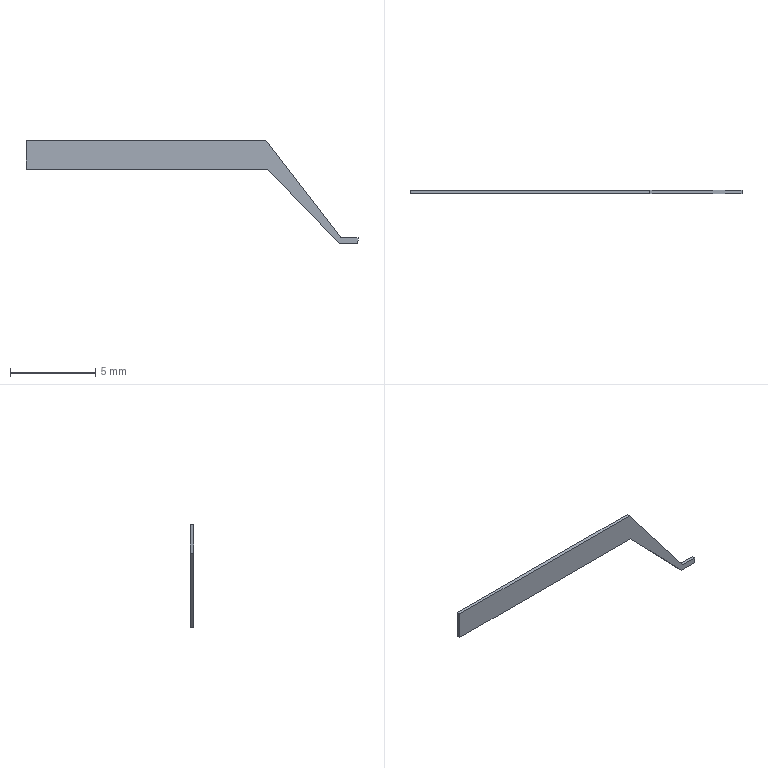Part | SolidWorks | features Extrusion 1 | 1 solid | 10 faces | box 19.5 x 0.2 x 6.07 mm | volume 5.761 mm3 | plane 10
STEP:
#1=CARTESIAN_POINT('',(0.,0.,-1.7));
#2=VERTEX_POINT('',#1);
#3=CARTESIAN_POINT('',(0.,0.,0.));
#4=VERTEX_POINT('',#3);
#5=CARTESIAN_POINT('',(0.,0.,0.));
#6=DIRECTION('',(0.,0.,1.));
#7=VECTOR('',#6,1000.);
#8=LINE('',#5,#7);
#9=EDGE_CURVE('',#2,#4,#8,.T.);
#10=ORIENTED_EDGE('',*,*,#9,.T.);
#11=CARTESIAN_POINT('',(0.,0.2,0.));
#12=VERTEX_POINT('',#11);
#13=CARTESIAN_POINT('',(0.,0.2,0.));
#14=DIRECTION('',(0.,-1.,0.));
#15=VECTOR('',#14,1000.);
#16=LINE('',#13,#15);
#17=EDGE_CURVE('',#12,#4,#16,.T.);
#18=ORIENTED_EDGE('',*,*,#17,.F.);
#19=CARTESIAN_POINT('',(0.,0.2,-1.7));
#20=VERTEX_POINT('',#19);
#21=CARTESIAN_POINT('',(0.,0.2,0.));
#22=DIRECTION('',(0.,0.,1.));
#23=VECTOR('',#22,1000.);
#24=LINE('',#21,#23);
#25=EDGE_CURVE('',#20,#12,#24,.T.);
#26=ORIENTED_EDGE('',*,*,#25,.F.);
#27=CARTESIAN_POINT('',(0.,0.2,-1.7));
#28=DIRECTION('',(0.,-1.,0.));
#29=VECTOR('',#28,1000.);
#30=LINE('',#27,#29);
#31=EDGE_CURVE('',#20,#2,#30,.T.);
#32=ORIENTED_EDGE('',*,*,#31,.T.);
#33=EDGE_LOOP('',(#10,#18,#26,#32));
#34=FACE_OUTER_BOUND('',#33,.T.);
#35=CARTESIAN_POINT('',(0.,0.2,0.));
#36=DIRECTION('',(1.,0.,0.));
#37=DIRECTION('',(0.,0.,-1.));
#38=AXIS2_PLACEMENT_3D('',#35,#36,#37);
#39=PLANE('',#38);
#40=ADVANCED_FACE('',(#34),#39,.F.);
#41=CARTESIAN_POINT('',(14.095,0.,0.));
#42=VERTEX_POINT('',#41);
#43=CARTESIAN_POINT('',(0.,0.,0.));
#44=DIRECTION('',(1.,0.,0.));
#45=VECTOR('',#44,1000.);
#46=LINE('',#43,#45);
#47=EDGE_CURVE('',#4,#42,#46,.T.);
#48=ORIENTED_EDGE('',*,*,#47,.T.);
#49=CARTESIAN_POINT('',(14.095,0.2,0.));
#50=VERTEX_POINT('',#49);
#51=CARTESIAN_POINT('',(14.095,0.2,0.));
#52=DIRECTION('',(0.,-1.,0.));
#53=VECTOR('',#52,1000.);
#54=LINE('',#51,#53);
#55=EDGE_CURVE('',#50,#42,#54,.T.);
#56=ORIENTED_EDGE('',*,*,#55,.F.);
#57=CARTESIAN_POINT('',(0.,0.2,0.));
#58=DIRECTION('',(1.,0.,0.));
#59=VECTOR('',#58,1000.);
#60=LINE('',#57,#59);
#61=EDGE_CURVE('',#12,#50,#60,.T.);
#62=ORIENTED_EDGE('',*,*,#61,.F.);
#63=ORIENTED_EDGE('',*,*,#17,.T.);
#64=EDGE_LOOP('',(#48,#56,#62,#63));
#65=FACE_OUTER_BOUND('',#64,.T.);
#66=CARTESIAN_POINT('',(0.,0.2,0.));
#67=DIRECTION('',(0.,0.,-1.));
#68=DIRECTION('',(-1.,0.,0.));
#69=AXIS2_PLACEMENT_3D('',#66,#67,#68);
#70=PLANE('',#69);
#71=ADVANCED_FACE('',(#65),#70,.F.);
#72=CARTESIAN_POINT('',(18.5,0.,-5.72));
#73=VERTEX_POINT('',#72);
#74=CARTESIAN_POINT('',(14.095,0.,0.));
#75=DIRECTION('',(0.6101,0.,-0.7923));
#76=VECTOR('',#75,1000.);
#77=LINE('',#74,#76);
#78=EDGE_CURVE('',#42,#73,#77,.T.);
#79=ORIENTED_EDGE('',*,*,#78,.T.);
#80=CARTESIAN_POINT('',(18.5,0.2,-5.72));
#81=VERTEX_POINT('',#80);
#82=CARTESIAN_POINT('',(18.5,0.2,-5.72));
#83=DIRECTION('',(0.,-1.,0.));
#84=VECTOR('',#83,1000.);
#85=LINE('',#82,#84);
#86=EDGE_CURVE('',#81,#73,#85,.T.);
#87=ORIENTED_EDGE('',*,*,#86,.F.);
#88=CARTESIAN_POINT('',(14.095,0.2,0.));
#89=DIRECTION('',(0.6101,0.,-0.7923));
#90=VECTOR('',#89,1000.);
#91=LINE('',#88,#90);
#92=EDGE_CURVE('',#50,#81,#91,.T.);
#93=ORIENTED_EDGE('',*,*,#92,.F.);
#94=ORIENTED_EDGE('',*,*,#55,.T.);
#95=EDGE_LOOP('',(#79,#87,#93,#94));
#96=FACE_OUTER_BOUND('',#95,.T.);
#97=CARTESIAN_POINT('',(14.095,0.2,0.));
#98=DIRECTION('',(-0.7923,0.,-0.6101));
#99=DIRECTION('',(-0.6101,0.,0.7923));
#100=AXIS2_PLACEMENT_3D('',#97,#98,#99);
#101=PLANE('',#100);
#102=ADVANCED_FACE('',(#96),#101,.F.);
#103=CARTESIAN_POINT('',(19.5,0.,-5.72));
#104=VERTEX_POINT('',#103);
#105=CARTESIAN_POINT('',(18.5,0.,-5.72));
#106=DIRECTION('',(1.,0.,0.));
#107=VECTOR('',#106,1000.);
#108=LINE('',#105,#107);
#109=EDGE_CURVE('',#73,#104,#108,.T.);
#110=ORIENTED_EDGE('',*,*,#109,.T.);
#111=CARTESIAN_POINT('',(19.5,0.2,-5.72));
#112=VERTEX_POINT('',#111);
#113=CARTESIAN_POINT('',(19.5,0.2,-5.72));
#114=DIRECTION('',(0.,-1.,0.));
#115=VECTOR('',#114,1000.);
#116=LINE('',#113,#115);
#117=EDGE_CURVE('',#112,#104,#116,.T.);
#118=ORIENTED_EDGE('',*,*,#117,.F.);
#119=CARTESIAN_POINT('',(18.5,0.2,-5.72));
#120=DIRECTION('',(1.,0.,0.));
#121=VECTOR('',#120,1000.);
#122=LINE('',#119,#121);
#123=EDGE_CURVE('',#81,#112,#122,.T.);
#124=ORIENTED_EDGE('',*,*,#123,.F.);
#125=ORIENTED_EDGE('',*,*,#86,.T.);
#126=EDGE_LOOP('',(#110,#118,#124,#125));
#127=FACE_OUTER_BOUND('',#126,.T.);
#128=CARTESIAN_POINT('',(18.5,0.2,-5.72));
#129=DIRECTION('',(0.,0.,-1.));
#130=DIRECTION('',(-1.,0.,0.));
#131=AXIS2_PLACEMENT_3D('',#128,#129,#130);
#132=PLANE('',#131);
#133=ADVANCED_FACE('',(#127),#132,.F.);
#134=CARTESIAN_POINT('',(19.5,0.,-6.07));
#135=VERTEX_POINT('',#134);
#136=CARTESIAN_POINT('',(19.5,0.,-5.72));
#137=DIRECTION('',(0.,0.,-1.));
#138=VECTOR('',#137,1000.);
#139=LINE('',#136,#138);
#140=EDGE_CURVE('',#104,#135,#139,.T.);
#141=ORIENTED_EDGE('',*,*,#140,.T.);
#142=CARTESIAN_POINT('',(19.5,0.2,-6.07));
#143=VERTEX_POINT('',#142);
#144=CARTESIAN_POINT('',(19.5,0.2,-6.07));
#145=DIRECTION('',(0.,-1.,0.));
#146=VECTOR('',#145,1000.);
#147=LINE('',#144,#146);
#148=EDGE_CURVE('',#143,#135,#147,.T.);
#149=ORIENTED_EDGE('',*,*,#148,.F.);
#150=CARTESIAN_POINT('',(19.5,0.2,-5.72));
#151=DIRECTION('',(0.,0.,-1.));
#152=VECTOR('',#151,1000.);
#153=LINE('',#150,#152);
#154=EDGE_CURVE('',#112,#143,#153,.T.);
#155=ORIENTED_EDGE('',*,*,#154,.F.);
#156=ORIENTED_EDGE('',*,*,#117,.T.);
#157=EDGE_LOOP('',(#141,#149,#155,#156));
#158=FACE_OUTER_BOUND('',#157,.T.);
#159=CARTESIAN_POINT('',(19.5,0.2,-5.72));
#160=DIRECTION('',(-1.,0.,0.));
#161=DIRECTION('',(0.,0.,1.));
#162=AXIS2_PLACEMENT_3D('',#159,#160,#161);
#163=PLANE('',#162);
#164=ADVANCED_FACE('',(#158),#163,.F.);
#165=CARTESIAN_POINT('',(18.405,0.,-6.07));
#166=VERTEX_POINT('',#165);
#167=CARTESIAN_POINT('',(18.405,0.,-6.07));
#168=DIRECTION('',(-1.,0.,0.));
#169=VECTOR('',#168,1000.);
#170=LINE('',#167,#169);
#171=EDGE_CURVE('',#135,#166,#170,.T.);
#172=ORIENTED_EDGE('',*,*,#171,.T.);
#173=CARTESIAN_POINT('',(18.405,0.2,-6.07));
#174=VERTEX_POINT('',#173);
#175=CARTESIAN_POINT('',(18.405,0.2,-6.07));
#176=DIRECTION('',(0.,-1.,0.));
#177=VECTOR('',#176,1000.);
#178=LINE('',#175,#177);
#179=EDGE_CURVE('',#174,#166,#178,.T.);
#180=ORIENTED_EDGE('',*,*,#179,.F.);
#181=CARTESIAN_POINT('',(18.405,0.2,-6.07));
#182=DIRECTION('',(-1.,0.,0.));
#183=VECTOR('',#182,1000.);
#184=LINE('',#181,#183);
#185=EDGE_CURVE('',#143,#174,#184,.T.);
#186=ORIENTED_EDGE('',*,*,#185,.F.);
#187=ORIENTED_EDGE('',*,*,#148,.T.);
#188=EDGE_LOOP('',(#172,#180,#186,#187));
#189=FACE_OUTER_BOUND('',#188,.T.);
#190=CARTESIAN_POINT('',(18.405,0.2,-6.07));
#191=DIRECTION('',(0.,0.,1.));
#192=DIRECTION('',(1.,0.,0.));
#193=AXIS2_PLACEMENT_3D('',#190,#191,#192);
#194=PLANE('',#193);
#195=ADVANCED_FACE('',(#189),#194,.F.);
#196=CARTESIAN_POINT('',(14.2,0.,-1.7));
#197=VERTEX_POINT('',#196);
#198=CARTESIAN_POINT('',(14.2,0.,-1.7));
#199=DIRECTION('',(-0.6934,0.,0.7206));
#200=VECTOR('',#199,1000.);
#201=LINE('',#198,#200);
#202=EDGE_CURVE('',#166,#197,#201,.T.);
#203=ORIENTED_EDGE('',*,*,#202,.T.);
#204=CARTESIAN_POINT('',(14.2,0.2,-1.7));
#205=VERTEX_POINT('',#204);
#206=CARTESIAN_POINT('',(14.2,0.2,-1.7));
#207=DIRECTION('',(0.,-1.,0.));
#208=VECTOR('',#207,1000.);
#209=LINE('',#206,#208);
#210=EDGE_CURVE('',#205,#197,#209,.T.);
#211=ORIENTED_EDGE('',*,*,#210,.F.);
#212=CARTESIAN_POINT('',(14.2,0.2,-1.7));
#213=DIRECTION('',(-0.6934,0.,0.7206));
#214=VECTOR('',#213,1000.);
#215=LINE('',#212,#214);
#216=EDGE_CURVE('',#174,#205,#215,.T.);
#217=ORIENTED_EDGE('',*,*,#216,.F.);
#218=ORIENTED_EDGE('',*,*,#179,.T.);
#219=EDGE_LOOP('',(#203,#211,#217,#218));
#220=FACE_OUTER_BOUND('',#219,.T.);
#221=CARTESIAN_POINT('',(14.2,0.2,-1.7));
#222=DIRECTION('',(0.7206,0.,0.6934));
#223=DIRECTION('',(0.6934,0.,-0.7206));
#224=AXIS2_PLACEMENT_3D('',#221,#222,#223);
#225=PLANE('',#224);
#226=ADVANCED_FACE('',(#220),#225,.F.);
#227=CARTESIAN_POINT('',(0.,0.,-1.7));
#228=DIRECTION('',(-1.,0.,0.));
#229=VECTOR('',#228,1000.);
#230=LINE('',#227,#229);
#231=EDGE_CURVE('',#197,#2,#230,.T.);
#232=ORIENTED_EDGE('',*,*,#231,.T.);
#233=ORIENTED_EDGE('',*,*,#31,.F.);
#234=CARTESIAN_POINT('',(0.,0.2,-1.7));
#235=DIRECTION('',(-1.,0.,0.));
#236=VECTOR('',#235,1000.);
#237=LINE('',#234,#236);
#238=EDGE_CURVE('',#205,#20,#237,.T.);
#239=ORIENTED_EDGE('',*,*,#238,.F.);
#240=ORIENTED_EDGE('',*,*,#210,.T.);
#241=EDGE_LOOP('',(#232,#233,#239,#240));
#242=FACE_OUTER_BOUND('',#241,.T.);
#243=CARTESIAN_POINT('',(0.,0.2,-1.7));
#244=DIRECTION('',(0.,0.,1.));
#245=DIRECTION('',(1.,0.,0.));
#246=AXIS2_PLACEMENT_3D('',#243,#244,#245);
#247=PLANE('',#246);
#248=ADVANCED_FACE('',(#242),#247,.F.);
#249=ORIENTED_EDGE('',*,*,#25,.T.);
#250=ORIENTED_EDGE('',*,*,#61,.T.);
#251=ORIENTED_EDGE('',*,*,#92,.T.);
#252=ORIENTED_EDGE('',*,*,#123,.T.);
#253=ORIENTED_EDGE('',*,*,#154,.T.);
#254=ORIENTED_EDGE('',*,*,#185,.T.);
#255=ORIENTED_EDGE('',*,*,#216,.T.);
#256=ORIENTED_EDGE('',*,*,#238,.T.);
#257=EDGE_LOOP('',(#249,#250,#251,#252,#253,#254,#255,#256));
#258=FACE_OUTER_BOUND('',#257,.T.);
#259=CARTESIAN_POINT('',(0.,0.2,0.));
#260=DIRECTION('',(0.,-1.,0.));
#261=DIRECTION('',(0.,0.,-1.));
#262=AXIS2_PLACEMENT_3D('',#259,#260,#261);
#263=PLANE('',#262);
#264=ADVANCED_FACE('',(#258),#263,.F.);
#265=ORIENTED_EDGE('',*,*,#9,.F.);
#266=ORIENTED_EDGE('',*,*,#231,.F.);
#267=ORIENTED_EDGE('',*,*,#202,.F.);
#268=ORIENTED_EDGE('',*,*,#171,.F.);
#269=ORIENTED_EDGE('',*,*,#140,.F.);
#270=ORIENTED_EDGE('',*,*,#109,.F.);
#271=ORIENTED_EDGE('',*,*,#78,.F.);
#272=ORIENTED_EDGE('',*,*,#47,.F.);
#273=EDGE_LOOP('',(#265,#266,#267,#268,#269,#270,#271,#272));
#274=FACE_OUTER_BOUND('',#273,.T.);
#275=CARTESIAN_POINT('',(0.,0.,0.));
#276=DIRECTION('',(0.,-1.,0.));
#277=DIRECTION('',(0.,0.,-1.));
#278=AXIS2_PLACEMENT_3D('',#275,#276,#277);
#279=PLANE('',#278);
#280=ADVANCED_FACE('',(#274),#279,.T.);
#281=CLOSED_SHELL('',(#40,#71,#102,#133,#164,#195,#226,#248,#264,#280));
#282=MANIFOLD_SOLID_BREP('',#281);
#283=CARTESIAN_POINT('',(0.,0.,0.));
#284=DIRECTION('',(0.,0.,1.));
#285=DIRECTION('',(1.,0.,0.));
#286=AXIS2_PLACEMENT_3D('',#283,#284,#285);
#287=(LENGTH_UNIT()NAMED_UNIT(*)SI_UNIT(.MILLI.,.METRE.));
#288=UNCERTAINTY_MEASURE_WITH_UNIT(LENGTH_MEASURE(0.00001),#287,'','');
#289=(NAMED_UNIT(*)PLANE_ANGLE_UNIT()SI_UNIT($,.RADIAN.));
#290=(NAMED_UNIT(*)SI_UNIT($,.STERADIAN.)SOLID_ANGLE_UNIT());
#291=(GEOMETRIC_REPRESENTATION_CONTEXT(3)GLOBAL_UNCERTAINTY_ASSIGNED_CONTEXT((#288))GLOBAL_UNIT_ASSIGNED_CONTEXT((#287,#289,#290))REPRESENTATION_CONTEXT('',''));
#292=ADVANCED_BREP_SHAPE_REPRESENTATION('',(#282,#286),#291);